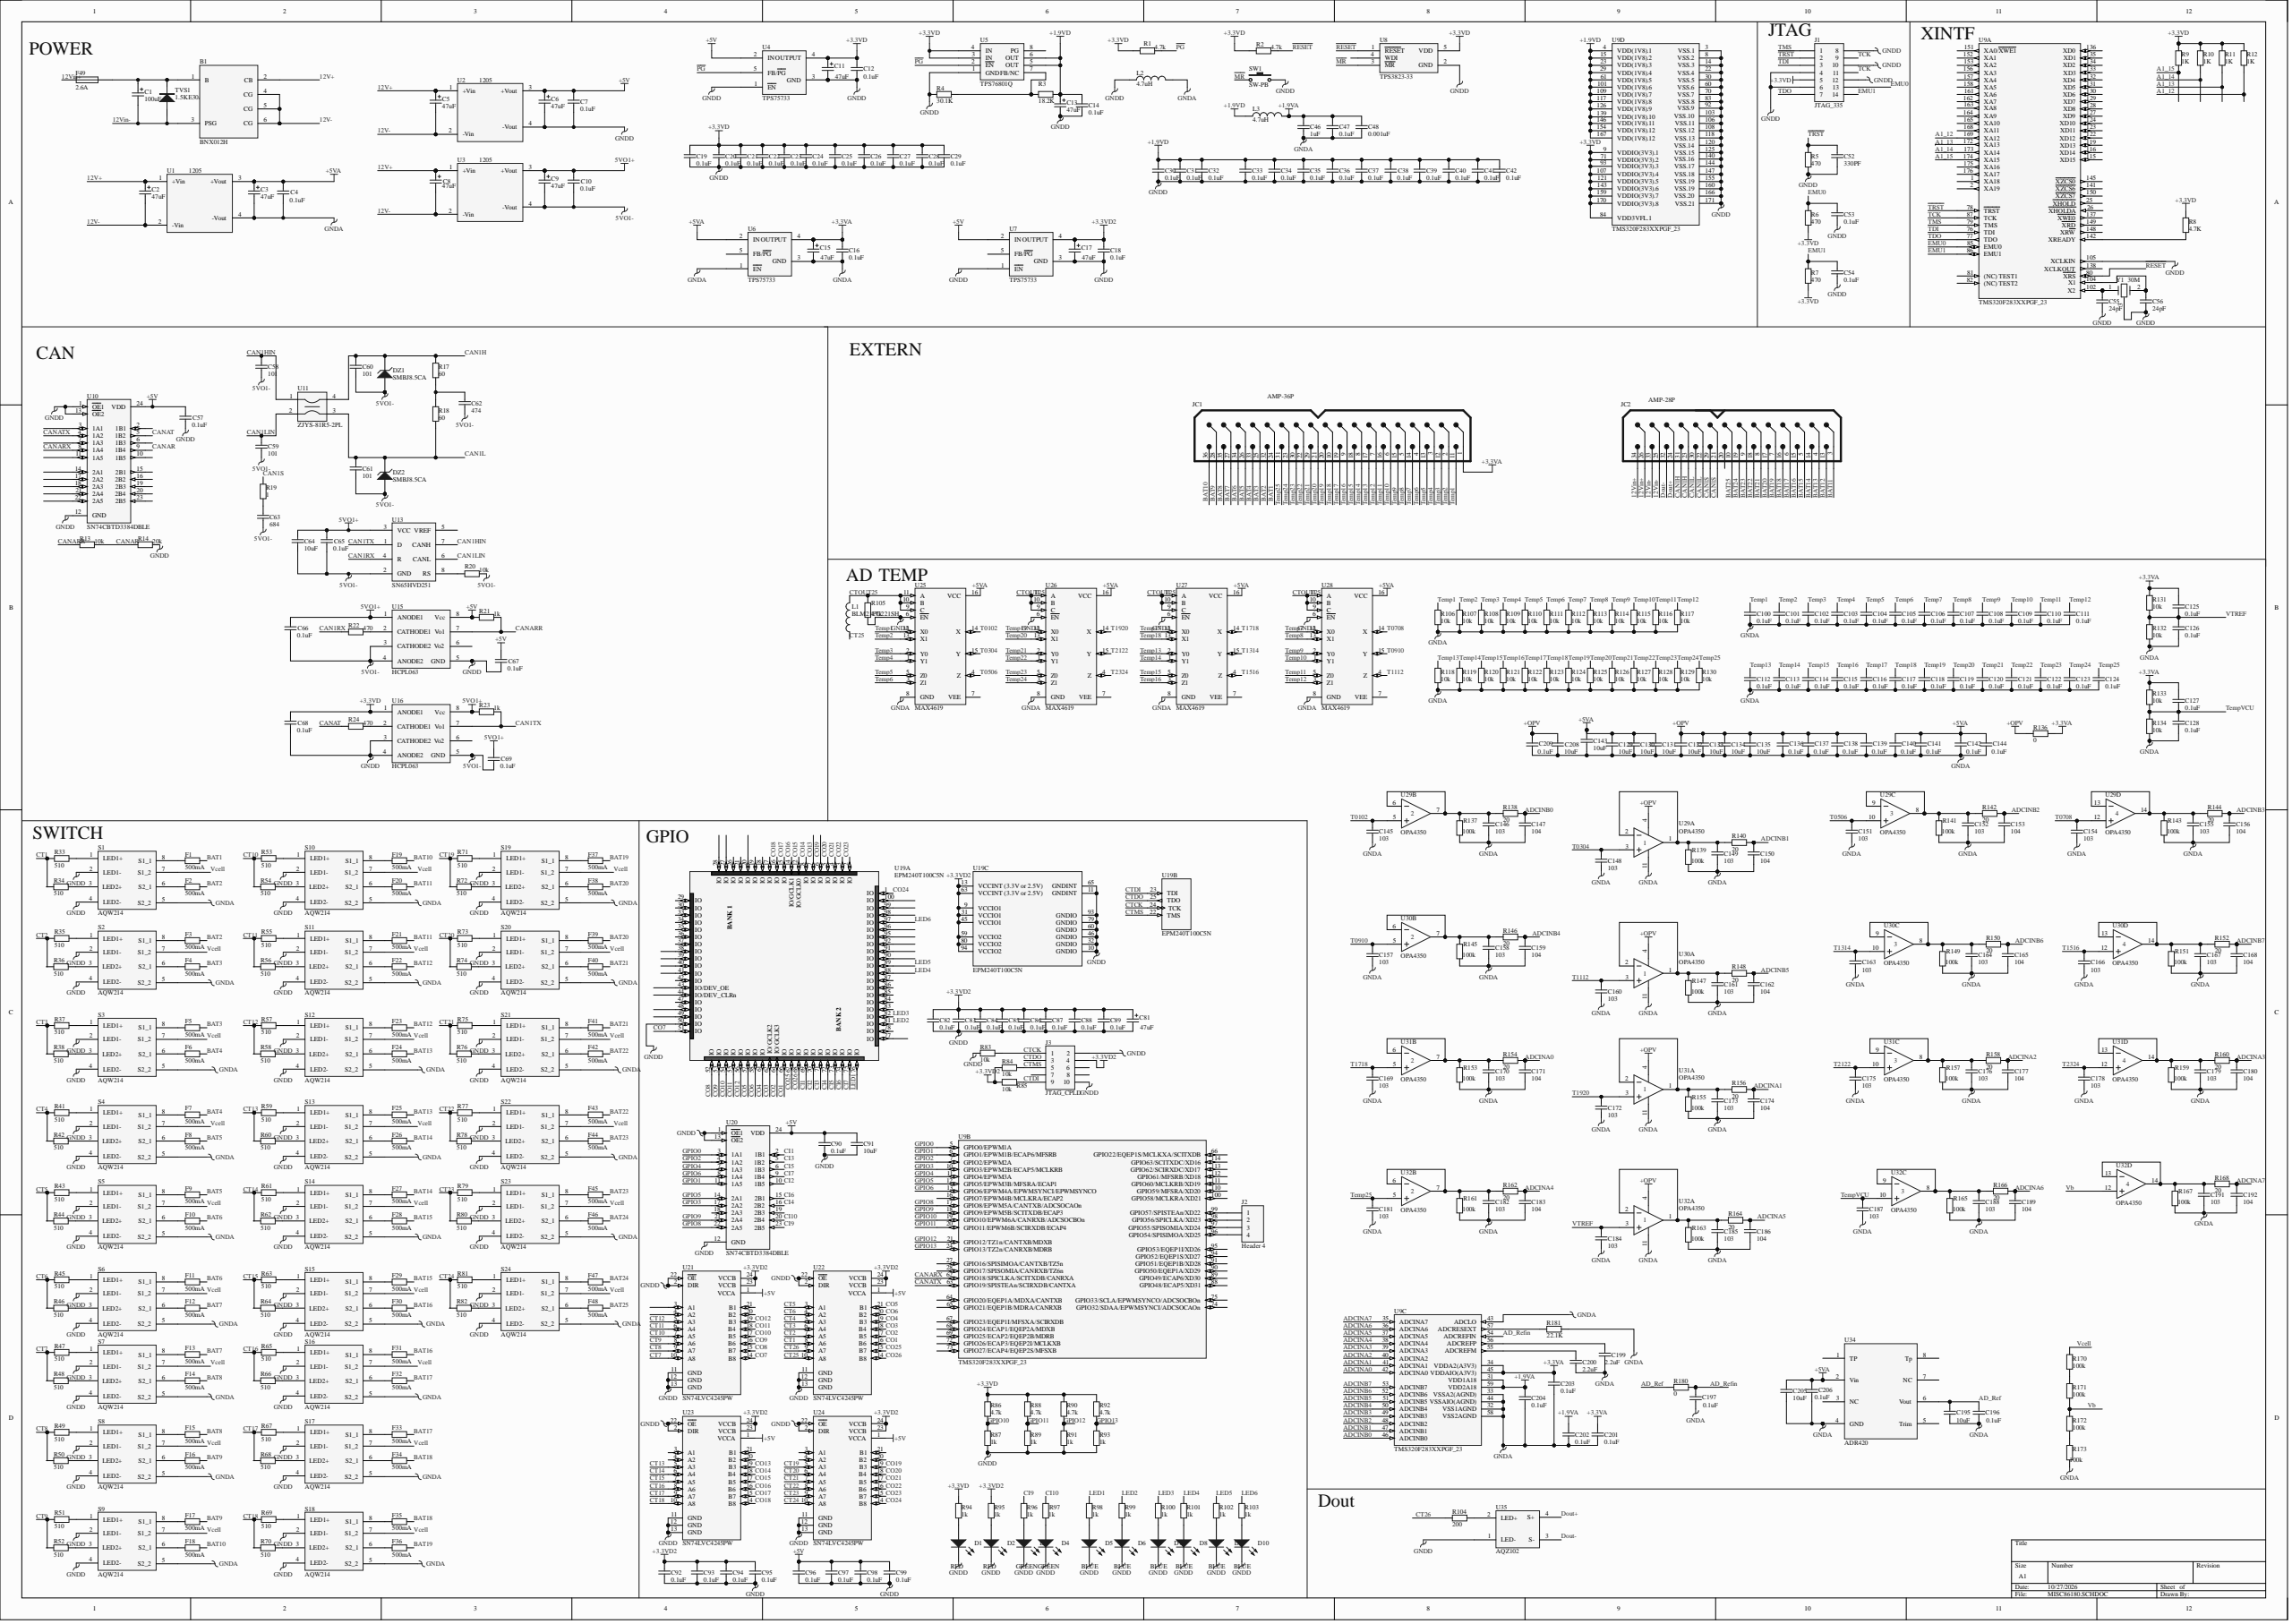Circuit board | Altium Designer | 475 parts | 355 nets
Bill of materials:
Comment,Description,Designator,Footprint,LibRef,Quantity
"BNX012H","","B1","BNX012H","BNX012H","1"
"Cap Pol3","Polarized Capacitor (Surface Mount)","C1, C2, C3, C5, C6, C8, C9, C11, C13, C15, C17, C81","TC7343-2917","Cap Pol3","12"
"Cap","Capacitor","C4, C7, C10, C125, C126, C127, C128","CR2012-0805","Cap","7"
"Cap","Capacitor","C12, C14, C16, C18, C19, C20, C21, C22, C23, C24, C25, C26, C27, C28, C29, C30, C31, C32, C33, C34, C35, C36, C37, C38, C39, C40, C41, C42, C47, C48, C52, C53, C54, C55, C56, C57, C58, C59, C60, C61, C62, C63, C65, C66, C67, C68, C69, C82, C83, C84, C85, C86, C87, C88, C89, C90, C92, C93, C94, C95, C96, C97, C98, C99, C100, C101, C102, C103, C104, C105, C106, C107, C108, C109, C110, C111, C112, C113, C114, C115, C116, C117, C118, C119, C120, C121, C122, C123, C124, C136, C137, C138, C139, C140, C141, C142, C144, C145, C146, C147, C148, C149, C150, C151, C152, C153, C154, C155, C156, C157, C158, C159, C160, C161, C162, C163, C164, C165, C166, C167, C168, C169, C170, C171, C172, C173, C174, C175, C176, C177, C178, C179, C180, C181, C182, C183, C184, C185, C186, C187, C188, C189, C191, C192, C196, C197, C199, C200, C201, C202, C203, C204, C206, C209","CR1608-0603","Cap","154"
"Cap","Capacitor","C46","1206","Cap","1"
"Cap","Capacitor","C64, C91, C129, C130, C131, C132, C133, C134, C135, C143, C195, C205, C208","CR3216-1206","Cap","13"
"RED","Typical YELLOW GaAs LED","D1, D2, D10","CR2012-0805","LED1","3"
"GREEN","Typical YELLOW GaAs LED","D3, D4","CR2012-0805","LED1","2"
"BLUE","Typical YELLOW GaAs LED","D5, D6, D7, D8, D9","CR2012-0805","LED1","5"
"SMBJ8.5CA","","DZ1, DZ2","AK_1B","AK1B","2"
"Res2","Resistor","F1, F2, F3, F4, F5, F6, F7, F8, F9, F10, F11, F12, F13, F14, F15, F16, F17, F18, F19, F20, F21, F22, F23, F24, F25, F26, F27, F28, F29, F30, F31, F32, F33, F34, F35, F36, F37, F38, F39, F40, F41, F42, F43, F44, F45, F46, F47, F48","CR6332-2512","Res2","48"
"2.6A","Fuse","F49","FUSE","FUSE1","1"
"JTAG_335","Header, 7-Pin, Dual row","J1","JTAG14","Header 7X2A","1"
"Header 4","Header, 4-Pin","J2","HDR1X4","Header 4","1"
"JTAG_CPLD","Header, 5-Pin, Dual row","J3","HDR2X5","Header 5X2","1"
"AMP-36P","","JC1","36P","AMP-36P","1"
"AMP-28P","","JC2","28P","AMP-28P","1"
"Inductor","Inductor","L1","INDC2012-0805","Inductor","1"
"Inductor","Inductor","L2, L3","CR3225-1210","Inductor","2"
"Res2","Resistor","R1, R2, R5, R6, R7, R8, R9, R10, R11, R12, R13, R14, R20, R21, R22, R23, R24, R83, R84, R85, R86, R87, R88, R89, R90, R91, R92, R93, R94, R95, R96, R97, R98, R99, R100, R101, R102, R103, R105, R137, R138, R139, R140, R141, R142, R143, R144, R145, R146, R147, R148, R149, R150, R151, R152, R153, R154, R155, R156, R157, R158, R159, R160, R161, R162, R163, R164, R165, R166, R167, R168, R181","CR1608-0603","Res2","72"
"Res2","Resistor","R3, R4, R17, R18, R19, R33, R34, R35, R36, R37, R38, R41, R42, R43, R44, R45, R46, R47, R48, R49, R50, R51, R52, R53, R54, R55, R56, R57, R58, R59, R60, R61, R62, R63, R64, R65, R66, R67, R68, R69, R70, R71, R72, R73, R74, R75, R76, R77, R78, R79, R80, R81, R82, R104, R106, R107, R108, R109, R110, R111, R112, R113, R114, R115, R116, R117, R118, R119, R120, R121, R122, R123, R124, R125, R126, R127, R128, R129, R130, R131, R132, R133, R134, R136, R170, R171, R172, R173, R180","CR2012-0805","Res2","89"
"AQW214","","S1, S2, S3, S4, S5, S6, S7, S8, S9, S10, S11, S12, S13, S14, S15, S16, S17, S18, S19, S20, S21, S22, S23, S24","AQW214","AQW214","24"
"SW-PB","Switch","SW1","SW_RESET","SW-PB","1"
"1.5KE30A","","TVS1","SB560","diode2","1"
"1205","","U1, U2, U3","DCDC_5W","DCDC","3"
"TPS75733","","U4, U6, U7","75733","TPS75733","3"
"TPS76801Q","","U5","D008","TPS76801Q","1"
"TPS3823-33","","U8","DBV005","TPS3823-33","1"
"TMS320F283XXPGF_23","","U9","QFP176NEW","TMS320F283XXPGF_23","1"
"SN74CBTD3384DBLE","10-Bit FET Bus Switch with Level Shifting","U10, U20","DBQ024","SN74CBTD3384DBLE","2"
"ZJYS-81R5-2PL","","U11","ZJYS","ZJYS-81R5-2PL","1"
"SN65HVD251","","U13","D008","SN65HVD251","1"
"HCPL063","","U15, U16","SO-G8","HCPL063","2"
"EPM240T100C5N","MAX II 2.5/3.3V CPLD, 80 I/Os, 100-Pin Plastic TQFP, Pb-Free, Commercial Temperature, Speed Grade 5","U19","TQFP100","EPM240T100C5N","1"
"SN74LVC4245PW","Octal Bus Transceiver and 3.3-V to 5-V Shifter with 3-State Outputs","U21, U22, U23, U24","WSO24","SN74LVC4245PW","4"
"MAX4619","Analog Multiplexer/Demultiplexer Triple 2-Channel","U25, U26, U27, U28","SO16","M74HC4053M1R","4"
"OPA4350","Quad Low-Power Operational Amplifier","U29, U30, U31, U32","751A-02","LM324D","4"
"ADR420","","U34","SO-G8","ADR421","1"
"AQZ102","","U35","AQZ102","AQZ","1"
"30M","Crystal","Y1","Oscillator","CRYSTAL","1"
Netlist (Protel format):
[
B1
BNX012H
BNX012H



]
[
C1
TC7343-2917
Cap Pol3



]
[
C2
TC7343-2917
Cap Pol3



]
[
C3
TC7343-2917
Cap Pol3



]
[
C4
CR2012-0805
Cap



]
[
C5
TC7343-2917
Cap Pol3



]
[
C6
TC7343-2917
Cap Pol3



]
[
C7
CR2012-0805
Cap



]
[
C8
TC7343-2917
Cap Pol3



]
[
C9
TC7343-2917
Cap Pol3



]
[
C10
CR2012-0805
Cap



]
[
C11
TC7343-2917
Cap Pol3



]
[
C12
CR1608-0603
Cap



]
[
C13
TC7343-2917
Cap Pol3



]
[
C14
CR1608-0603
Cap



]
[
C15
TC7343-2917
Cap Pol3



]
[
C16
CR1608-0603
Cap



]
[
C17
TC7343-2917
Cap Pol3



]
[
C18
CR1608-0603
Cap



]
[
C19
CR1608-0603
Cap



]
[
C20
CR1608-0603
Cap



]
[
C21
CR1608-0603
Cap



]
[
C22
CR1608-0603
Cap



]
[
C23
CR1608-0603
Cap



]
[
C24
CR1608-0603
Cap



]
[
C25
CR1608-0603
Cap



]
[
C26
CR1608-0603
Cap



]
[
C27
CR1608-0603
Cap



]
[
C28
CR1608-0603
Cap



]
[
C29
CR1608-0603
Cap



]
[
C30
CR1608-0603
Cap



]
[
C31
CR1608-0603
Cap



]
[
C32
CR1608-0603
Cap



]
[
C33
CR1608-0603
Cap



]
[
C34
CR1608-0603
Cap



]
[
C35
CR1608-0603
Cap



]
[
C36
CR1608-0603
Cap



]
[
C37
CR1608-0603
Cap



]
[
C38
CR1608-0603
Cap



]
[
C39
CR1608-0603
Cap



]
[
C40
CR1608-0603
Cap



]
[
C41
CR1608-0603
Cap



]
[
C42
CR1608-0603
Cap



]
[
C46
1206
Cap



]
[
C47
CR1608-0603
Cap



]
[
C48
CR1608-0603
Cap



]
[
C52
CR1608-0603
Cap



]
[
C53
CR1608-0603
Cap



]
[
C54
CR1608-0603
Cap



]
[
C55
CR1608-0603
Cap



]
[
C56
CR1608-0603
Cap



]
[
C57
CR1608-0603
Cap



]
[
C58
CR1608-0603
Cap



]
[
C59
CR1608-0603
Cap



]
[
C60
CR1608-0603
Cap



]
[
C61
CR1608-0603
Cap



]
[
C62
CR1608-0603
Cap



]
[
C63
CR1608-0603
Cap



]
[
C64
CR3216-1206
Cap



]
[
C65
CR1608-0603
Cap



]
[
C66
CR1608-0603
Cap



]
[
C67
CR1608-0603
Cap



]
[
C68
CR1608-0603
Cap



]
[
C69
CR1608-0603
Cap



]
[
C81
TC7343-2917
Cap Pol3



]
[
C82
CR1608-0603
Cap



]
[
C83
CR1608-0603
Cap



]
[
C84
CR1608-0603
Cap



]
[
C85
CR1608-0603
Cap



]
[
C86
CR1608-0603
Cap



]
[
C87
CR1608-0603
Cap



]
[
C88
CR1608-0603
Cap



]
[
C89
CR1608-0603
Cap



]
[
C90
CR1608-0603
Cap



]
[
C91
CR3216-1206
Cap



]
[
C92
CR1608-0603
Cap



]
[
C93
CR1608-0603
Cap



]
[
C94
CR1608-0603
Cap



]
[
C95
CR1608-0603
Cap



]
[
C96
CR1608-0603
Cap



]
[
C97
CR1608-0603
Cap



]
[
C98
CR1608-0603
Cap



]
[
C99
CR1608-0603
Cap



]
[
C100
CR1608-0603
Cap



]
[
C101
CR1608-0603
Cap



]
[
C102
CR1608-0603
Cap



]
[
C103
CR1608-0603
Cap



]
[
C104
CR1608-0603
Cap



]
[
C105
CR1608-0603
Cap



]
[
C106
CR1608-0603
Cap



]
[
C107
CR1608-0603
Cap



]
[
C108
CR1608-0603
Cap



]
[
C109
CR1608-0603
Cap



]
[
C110
CR1608-0603
Cap



]
[
C111
CR1608-0603
Cap



]
[
C112
CR1608-0603
Cap



]
[
C113
CR1608-0603
Cap



]
[
C114
CR1608-0603
Cap



]
[
C115
CR1608-0603
Cap



]
[
C116
CR1608-0603
Cap



]
[
C117
CR1608-0603
Cap



]
[
C118
CR1608-0603
Cap



]
[
C119
CR1608-0603
Cap



]
[
C120
CR1608-0603
Cap



]
[
C121
CR1608-0603
Cap



]
[
C122
CR1608-0603
Cap



]
[
C123
CR1608-0603
Cap



]
[
C124
CR1608-0603
Cap



]
[
C125
CR2012-0805
Cap



]
[
C126
CR2012-0805
Cap



]
[
C127
CR2012-0805
Cap



]
[
C128
CR2012-0805
Cap



]
[
C129
CR3216-1206
Cap



]
[
C130
CR3216-1206
Cap



]
[
C131
CR3216-1206
Cap



]
[
C132
CR3216-1206
Cap



]
[
C133
CR3216-1206
Cap



]
[
C134
CR3216-1206
Cap



]
[
C135
CR3216-1206
Cap



]
[
C136
CR1608-0603
Cap



]
[
C137
CR1608-0603
Cap



]
[
C138
CR1608-0603
Cap



]
[
C139
CR1608-0603
Cap



]
[
C140
CR1608-0603
Cap



]
[
C141
CR1608-0603
Cap



]
[
C142
CR1608-0603
Cap



]
[
C143
CR3216-1206
Cap



]
[
C144
CR1608-0603
Cap



]
[
C145
CR1608-0603
Cap



]
[
C146
CR1608-0603
Cap



]
[
C147
CR1608-0603
Cap



]
[
C148
CR1608-0603
Cap



]
[
C149
CR1608-0603
Cap



]
[
C150
CR1608-0603
Cap



]
[
C151
CR1608-0603
Cap



]
[
C152
CR1608-0603
Cap



]
[
C153
CR1608-0603
Cap



]
[
C154
CR1608-0603
Cap



]
[
C155
CR1608-0603
Cap



]
[
C156
CR1608-0603
Cap



]
[
C157
CR1608-0603
Cap



]
[
C158
CR1608-0603
Cap



]
[
C159
CR1608-0603
Cap



]
[
C160
CR1608-0603
Cap



]
[
C161
CR1608-0603
Cap



]
[
C162
CR1608-0603
Cap



]
[
C163
CR1608-0603
Cap



]
[
C164
CR1608-0603
Cap



]
[
C165
CR1608-0603
Cap



]
[
C166
CR1608-0603
Cap



]
[
C167
CR1608-0603
Cap



]
[
C168
CR1608-0603
Cap



]
[
C169
CR1608-0603
Cap



]
[
C170
CR1608-0603
Cap



]
[
C171
CR1608-0603
Cap



]
[
C172
CR1608-0603
Cap



]
[
C173
CR1608-0603
Cap



]
[
C174
CR1608-0603
Cap



]
[
C175
CR1608-0603
Cap



]
[
C176
CR1608-0603
Cap



]
[
C177
CR1608-0603
Cap



]
[
C178
CR1608-0603
Cap



]
[
C179
CR1608-0603
Cap



]
[
C180
CR1608-0603
Cap



]
[
C181
CR1608-0603
Cap



]
[
C182
CR1608-0603
Cap



]
[
C183
CR1608-0603
Cap



]
[
C184
CR1608-0603
Cap



]
[
C185
CR1608-0603
Cap



]
[
C186
CR1608-0603
Cap



]
[
C187
CR1608-0603
Cap



]
[
C188
CR1608-0603
Cap



]
[
C189
CR1608-0603
Cap



]
[
C191
CR1608-0603
Cap



]
[
C192
CR1608-0603
Cap



]
[
C195
CR3216-1206
Cap



]
[
C196
CR1608-0603
Cap



]
[
C197
CR1608-0603
Cap



]
[
C199
CR1608-0603
Cap



]
[
C200
CR1608-0603
Cap



]
[
C201
CR1608-0603
Cap



]
[
C202
CR1608-0603
Cap



]
[
C203
CR1608-0603
Cap



]
[
C204
CR1608-0603
Cap



]
[
C205
CR3216-1206
Cap



]
[
C206
CR1608-0603
Cap



]
[
C208
CR3216-1206
Cap



]
[
C209
CR1608-0603
Cap



]
[
D1
CR2012-0805
RED



]
[
D2
CR2012-0805
RED



]
[
D3
CR2012-0805
GREEN



]
[
D4
CR2012-0805
GREEN



]
[
D5
CR2012-0805
BLUE



]
[
D6
CR2012-0805
BLUE



]
[
D7
CR2012-0805
BLUE



]
[
D8
CR2012-0805
BLUE



]
[
D9
CR2012-0805
BLUE



]
[
D10
CR2012-0805
RED



]
[
DZ1
AK_1B
SMBJ8.5CA



]
[
DZ2
AK_1B
SMBJ8.5CA



]
[
F1
CR6332-2512
Res2



]
[
F2
CR6332-2512
Res2



]
[
F3
CR6332-2512
Res2



]
[
F4
CR6332-2512
Res2



]
[
F5
CR6332-2512
Res2



]
[
F6
CR6332-2512
Res2



]
[
F7
CR6332-2512
Res2



]
[
F8
CR6332-2512
Res2



]
[
F9
CR6332-2512
Res2



]
[
F10
CR6332-2512
Res2



]
[
F11
CR6332-2512
Res2



]
[
F12
CR6332-2512
Res2



]
[
F13
CR6332-2512
Res2



]
[
F14
CR6332-2512
Res2



]
[
F15
CR6332-2512
Res2



]
[
F16
CR6332-2512
Res2



]
[
F17
CR6332-2512
Res2



]
[
F18
CR6332-2512
Res2



]
[
F19
CR6332-2512
Res2



]
[
F20
CR6332-2512
Res2



]
[
F21
CR6332-2512
Res2



]
[
F22
CR6332-2512
Res2



]
[
F23
CR6332-2512
Res2



]
[
F24
CR6332-2512
Res2



]
[
F25
CR6332-2512
Res2



]
[
F26
CR6332-2512
Res2



]
[
F27
CR6332-2512
Res2



]
[
F28
CR6332-2512
Res2



]
[
F29
CR6332-2512
Res2



]
[
F30
CR6332-2512
Res2



]
[
F31
CR6332-2512
Res2



]
[
F32
CR6332-2512
Res2



]
[
F33
CR6332-2512
Res2



]
[
F34
CR6332-2512
Res2



]
[
F35
CR6332-2512
Res2



]
[
F36
CR6332-2512
Res2



]
[
F37
CR6332-2512
Res2



]
[
F38
CR6332-2512
Res2



]
[
F39
CR6332-2512
Res2



]
[
F40
CR6332-2512
Res2



]
[
F41
CR6332-2512
Res2



]
[
F42
CR6332-2512
Res2



]
[
F43
CR6332-2512
Res2



]
[
F44
CR6332-2512
Res2



]
[
F45
CR6332-2512
Res2



]
[
F46
CR6332-2512
Res2



]
[
F47
CR6332-2512
Res2



]
[
F48
CR6332-2512
Res2



]
[
F49
FUSE
2.6A



]
[
J1
JTAG14
JTAG_335



]
[
J2
HDR1X4
Header 4



]
[
J3
HDR2X5
JTAG_CPLD



]
[
JC1
36P
AMP-36P



]
[
JC2
28P
AMP-28P



]
[
L1
INDC2012-0805
Inductor



]
[
L2
CR3225-1210
Inductor



]
[
L3
CR3225-1210
Inductor



]
[
R1
CR1608-0603
Res2



]
[
R2
CR1608-0603
Res2



]
[
R3
CR2012-0805
Res2



]
[
R4
CR2012-0805
Res2



]
[
R5
CR1608-0603
Res2



]
[
R6
CR1608-0603
Res2



]
[
R7
CR1608-0603
Res2



]
[
R8
CR1608-0603
Res2



]
[
R9
CR1608-0603
Res2



]
[
R10
CR1608-0603
Res2



]
[
R11
CR1608-0603
Res2



]
[
R12
CR1608-0603
Res2



]
[
R13
CR1608-0603
Res2



]
[
R14
CR1608-0603
Res2



]
[
R17
CR2012-0805
Res2



]
[
R18
CR2012-0805
Res2



]
[
R19
CR2012-0805
Res2



]
[
R20
CR1608-0603
Res2



]
[
R21
CR1608-0603
Res2



]
[
R22
CR1608-0603
Res2



]
[
R23
CR1608-0603
Res2



]
[
R24
CR1608-0603
Res2



]
[
R33
CR2012-0805
Res2



]
[
R34
CR2012-0805
Res2



]
[
R35
CR2012-0805
Res2



]
[
R36
CR2012-0805
Res2



]
[
R37
CR2012-0805
Res2



]
[
R38
CR2012-0805
Res2



]
[
R41
CR2012-0805
Res2



]
[
R42
CR2012-0805
Res2



]
[
R43
CR2012-0805
Res2



]
[
R44
CR2012-0805
Res2



]
[
R45
CR2012-0805
Res2



]
[
R46
CR2012-0805
Res2



]
[
R47
CR2012-0805
Res2



]
[
R48
CR2012-0805
Res2



]
[
R49
CR2012-0805
Res2



]
[
R50
CR2012-0805
Res2



]
[
R51
CR2012-0805
Res2



]
[
R52
CR2012-0805
Res2



]
[
R53
CR2012-0805
Res2



]
[
R54
CR2012-0805
Res2



]
[
R55
CR2012-0805
Res2



]
[
R56
CR2012-0805
Res2



]
[
R57
CR2012-0805
Res2



]
[
R58
CR2012-0805
Res2



]
[
R59
CR2012-0805
Res2



]
[
R60
CR2012-0805
Res2



]
[
R61
CR2012-0805
Res2



]
[
R62
CR2012-0805
Res2



]
[
R63
CR2012-0805
Res2



]
[
R64
CR2012-0805
Res2



]
[
R65
CR2012-0805
Res2



]
[
R66
CR2012-0805
Res2



]
[
R67
CR2012-0805
Res2



]
[
R68
CR2012-0805
Res2



]
[
R69
CR2012-0805
Res2



]
[
R70
CR2012-0805
Res2



]
[
R71
CR2012-0805
Res2



]
[
R72
CR2012-0805
Res2



]
[
R73
CR2012-0805
Res2



]
[
R74
CR2012-0805
Res2



]
[
R75
CR2012-0805
Res2



]
[
R76
CR2012-0805
Res2



]
[
R77
CR2012-0805
Res2



]
[
R78
CR2012-0805
Res2



]
[
R79
CR2012-0805
Res2



]
[
R80
CR2012-0805
Res2



]
[
R81
CR2012-0805
Res2



]
[
R82
CR2012-0805
Res2



]
[
R83
CR1608-0603
Res2



]
[
R84
CR1608-0603
Res2



]
[
R85
CR1608-0603
Res2



]
[
R86
CR1608-0603
Res2



]
[
R87
CR1608-0603
Res2



]
[
R88
CR1608-0603
Res2



]
[
R89
CR1608-0603
Res2



]
[
R90
CR1608-0603
Res2



]
[
R91
CR1608-0603
Res2



]
[
R92
CR1608-0603
Res2



]
[
R93
CR1608-0603
Res2



]
[
R94
CR1608-0603
Res2



]
[
R95
CR1608-0603
Res2



]
[
R96
CR1608-0603
Res2



]
[
R97
CR1608-0603
Res2



]
[
R98
CR1608-0603
Res2



]
[
R99
CR1608-0603
Res2



]
[
R100
CR1608-0603
Res2



]
[
R101
CR1608-0603
Res2



]
[
R102
CR1608-0603
Res2



]
[
R103
CR1608-0603
Res2



]
[
R104
CR2012-0805
Res2



]
[
R105
CR1608-0603
Res2



]
[
R106
CR2012-0805
Res2



]
[
R107
CR2012-0805
Res2



]
[
R108
CR2012-0805
Res2



]
[
R109
CR2012-0805
Res2



]
[
R110
CR2012-0805
Res2



]
[
R111
CR2012-0805
Res2



]
[
R112
CR2012-0805
Res2



]
[
R113
CR2012-0805
Res2



]
[
R114
CR2012-0805
Res2



]
[
R115
CR2012-0805
Res2



]
[
R116
CR2012-0805
Res2



]
[
R117
CR2012-0805
Res2



]
[
R118
CR2012-0805
Res2



]
[
R119
CR2012-0805
Res2



]
[
R120
CR2012-0805
Res2



]
[
R121
CR2012-0805
Res2



]
[
R122
CR2012-0805
Res2



]
[
R123
CR2012-0805
Res2



]
[
R124
CR2012-0805
Res2



]
[
R125
CR2012-0805
Res2



]
[
R126
CR2012-0805
Res2



]
[
R127
CR2012-0805
Res2



]
[
R128
CR2012-0805
Res2



]
[
R129
CR2012-0805
Res2



]
[
R130
CR2012-0805
Res2



]
[
R131
CR2012-0805
Res2



]
[
R132
CR2012-0805
Res2



]
[
R133
CR2012-0805
Res2



]
[
R134
CR2012-0805
Res2



]
[
R136
CR2012-0805
Res2



]
[
R137
CR1608-0603
Res2



]
[
R138
CR1608-0603
Res2



]
[
R139
CR1608-0603
Res2



]
[
R140
CR1608-0603
Res2



]
[
R141
CR1608-0603
Res2



]
[
R142
CR1608-0603
Res2



]
[
R143
CR1608-0603
Res2



]
[
R144
CR1608-0603
Res2



]
[
R145
CR1608-0603
Res2



]
[
R146
CR1608-0603
Res2



]
[
R147
CR1608-0603
Res2



]
[
R148
CR1608-0603
Res2



]
[
R149
CR1608-0603
Res2



]
[
R150
CR1608-0603
Res2



]
[
R151
CR1608-0603
Res2



]
[
R152
CR1608-0603
Res2



]
[
R153
CR1608-0603
Res2



]
[
R154
CR1608-0603
Res2



]
[
R155
CR1608-0603
Res2



]
[
R156
CR1608-0603
Res2



]
[
R157
CR1608-0603
Res2



]
[
R158
CR1608-0603
Res2



]
[
R159
CR1608-0603
Res2



]
[
R160
CR1608-0603
Res2



]
[
R161
CR1608-0603
Res2



]
[
R162
CR1608-0603
Res2



]
[
R163
CR1608-0603
Res2



]
[
R164
CR1608-0603
Res2



]
[
R165
CR1608-0603
Res2



]
[
R166
CR1608-0603
Res2



]
[
R167
CR1608-0603
Res2



]
[
R168
CR1608-0603
Res2



]
[
R170
CR2012-0805
Res2



]
[
R171
CR2012-0805
Res2



]
[
R172
CR2012-0805
Res2



]
[
R173
CR2012-0805
Res2



]
[
R180
CR2012-0805
Res2



]
[
R181
CR1608-0603
Res2



]
[
S1
AQW214
AQW214



]
[
S2
AQW214
AQW214



]
[
S3
AQW214
AQW214



]
[
S4
AQW214
AQW214



]
[
S5
AQW214
AQW214



]
[
S6
AQW214
AQW214



]
[
S7
AQW214
AQW214



]
[
S8
AQW214
AQW214



]
[
S9
AQW214
AQW214



]
[
S10
AQW214
AQW214



]
[
S11
AQW214
AQW214



]
[
S12
AQW214
AQW214



]
[
S13
AQW214
AQW214



]
[
S14
AQW214
AQW214



]
[
S15
AQW214
AQW214



]
[
S16
AQW214
AQW214



]
[
S17
AQW214
AQW214



]
[
S18
AQW214
AQW214



]
[
S19
AQW214
AQW214



]
[
S20
AQW214
AQW214



]
[
S21
AQW214
AQW214



]
[
S22
AQW214
AQW214



]
[
S23
AQW214
AQW214



]
[
S24
AQW214
AQW214



]
[
SW1
SW_RESET
SW-PB



]
[
TVS1
SB560
1.5KE30A



]
[
U1
DCDC_5W
1205



]
[
U2
DCDC_5W
1205



]
[
U3
DCDC_5W
1205



]
[
U4
75733
TPS75733



]
[
U5
D008
TPS76801Q



]
[
U6
75733
TPS75733



]
[
U7
75733
TPS75733



]
[
U8
DBV005
TPS3823-33



]
[
U9
QFP176NEW
TMS320F283XXPGF_23



]
[
U10
DBQ024
SN74CBTD3384DBLE



]
[
U11
ZJYS
ZJYS-81R5-2PL



]
[
U13
D008
SN65HVD251



]
[
U15
SO-G8
HCPL063



]
[
U16
SO-G8
HCPL063



]
[
U19
TQFP100
EPM240T100C5N



]
[
U20
DBQ024
SN74CBTD3384DBLE



]
[
U21
WSO24
SN74LVC4245PW



]
[
U22
WSO24
SN74LVC4245PW



]
[
U23
WSO24
SN74LVC4245PW



]
[
U24
WSO24
SN74LVC4245PW



]
[
U25
SO16
MAX4619



]
[
U26
SO16
MAX4619



]
[
U27
SO16
MAX4619



]
[
U28
SO16
MAX4619



]
[
U29
751A-02
OPA4350



]
[
U30
751A-02
OPA4350



]
[
U31
751A-02
OPA4350



]
[
U32
751A-02
OPA4350



]
[
U34
SO-G8
ADR420



]
[
U35
AQZ102
AQZ102



]
[
Y1
Oscillator
30M



]
(
VTREF
C125-1
C126-2
C184-2
R131-2
R132-1
U32-3
)
(
Vcell
R170-1
S1-7
S2-7
S3-7
S4-7
S5-7
S6-7
S7-7
S8-7
S9-7
S10-7
S11-7
S12-7
S13-7
S14-7
S15-7
S16-7
S17-7
S18-7
S19-7
S20-7
S21-7
S22-7
S23-7
S24-7
)
(
Vb
R171-2
R172-1
U32-12
)
(
TMS
J1-1
U9-79
)
(
TempVCU
C127-1
C128-2
C187-2
R133-2
R134-1
U32-10
)
(
Temp25
C124-2
C181-2
JC1-31
R130-1
U32-5
)
(
Temp24
C123-2
JC1-23
R129-1
U26-3
)
(
Temp23
C122-2
JC1-30
R128-1
U26-5
)
(
Temp22
C121-2
JC1-22
R127-1
U26-1
)
(
Temp21
C120-2
JC1-29
R126-1
U26-2
)
(
Temp20
C119-2
JC1-21
R125-1
U26-13
)
(
Temp19
C118-2
JC1-20
R124-1
U26-12
)
(
Temp18
C117-2
JC1-10
R123-1
U27-13
)
(
Temp17
C116-2
JC1-19
R122-1
U27-12
)
(
Temp16
C115-2
JC1-9
R121-1
U27-3
)
(
Temp15
C114-2
JC1-18
R120-1
U27-5
)
(
Temp14
C113-2
JC1-8
R119-1
U27-1
)
(
Temp13
C112-2
JC1-17
R118-1
U27-2
)
(
Temp12
C111-2
JC1-7
R117-1
U28-3
)
(
Temp11
C110-2
JC1-16
R116-1
U28-5
)
(
Temp10
C109-2
JC1-6
R115-1
U28-1
)
(
Temp9
C108-2
JC1-15
R114-1
U28-2
)
(
Temp8
C107-2
JC1-5
R113-1
U28-13
)
(
Temp7
C106-2
JC1-14
R112-1
U28-12
)
(
Temp6
C105-2
JC1-4
R111-1
U25-3
)
(
Temp5
C104-2
JC1-13
R110-1
U25-5
)
(
Temp4
C103-2
JC1-3
R109-1
U25-1
)
(
Temp3
C102-2
JC1-12
R108-1
U25-2
)
(
Temp2
C101-2
JC1-2
R107-1
U25-13
)
(
Temp1
C100-2
JC1-11
R106-1
U25-12
)
(
TDO
J1-7
U9-77
)
(
TDI
J1-3
U9-76
)
(
TCK
J1-9
J1-11
U9-87
)
(
T\R\S\T\
C52-2
J1-2
R5-2
U9-78
)
(
T2324
C178-2
U26-4
U31-12
)
(
T2122
C175-2
U26-15
U31-10
)
(
T1920
C172-2
U26-14
U31-3
)
(
T1718
C169-2
U27-14
U31-5
)
(
T1516
C166-2
U27-4
U30-12
)
(
T1314
C163-2
U27-15
U30-10
)
(
T1112
C160-2
U28-4
U30-3
)
(
T0910
C157-2
U28-15
U30-5
)
(
T0708
C154-2
U28-14
U29-12
)
(
T0506
C151-2
U25-4
U29-10
)
(
T0304
C148-2
U25-15
U29-3
)
(
T0102
C145-2
U25-14
U29-5
)
(
R\E\S\E\T\
R2-2
U8-1
U9-80
)
(
P\G\
R1-2
U4-5
U5-2
)
(
NetR181_1
R181-1
U9-57
)
(
NetR172_2
R172-2
R173-1
)
(
NetR170_2
R170-2
R171-1
)
(
NetR104_1
R104-1
U35-2
)
(
NetR82_1
R82-1
S24-3
)
(
NetR81_1
R81-1
S24-1
)
(
NetR80_1
R80-1
S23-3
)
(
NetR79_1
R79-1
S23-1
)
(
NetR78_1
R78-1
S22-3
)
(
NetR77_1
R77-1
S22-1
)
(
NetR76_1
R76-1
S21-3
)
(
NetR75_1
R75-1
S21-1
)
(
NetR74_1
R74-1
S20-3
)
(
NetR73_1
R73-1
S20-1
)
(
NetR72_1
R72-1
S19-3
)
(
NetR71_1
R71-1
S19-1
)
(
NetR70_1
R70-1
S18-3
)
(
NetR69_1
R69-1
S18-1
)
(
NetR68_1
R68-1
S17-3
)
(
NetR67_1
R67-1
S17-1
)
(
NetR66_1
R66-1
S16-3
)
(
NetR65_1
R65-1
S16-1
)
(
NetR64_1
R64-1
S15-3
)
(
NetR63_1
R63-1
S15-1
)
(
NetR62_1
R62-1
S14-3
)
(
NetR61_1
R61-1
S14-1
)
(
NetR60_1
R60-1
S13-3
)
(
NetR59_1
R59-1
S13-1
)
(
NetR58_1
R58-1
S12-3
)
(
NetR57_1
R57-1
S12-1
)
(
NetR56_1
R56-1
S11-3
)
(
NetR55_1
R55-1
S11-1
)
(
NetR54_1
R54-1
S10-3
)
(
NetR53_1
R53-1
S10-1
)
(
NetR52_1
R52-1
S9-3
)
(
NetR51_1
R51-1
S9-1
)
(
NetR50_1
R50-1
S8-3
)
(
NetR49_1
R49-1
S8-1
)
(
NetR48_1
R48-1
S7-3
)
(
NetR47_1
R47-1
S7-1
)
(
NetR46_1
R46-1
S6-3
)
(
NetR45_1
R45-1
S6-1
)
(
NetR44_1
R44-1
S5-3
)
(
NetR43_1
R43-1
S5-1
)
(
NetR42_1
R42-1
S4-3
)
(
NetR41_1
R41-1
S4-1
)
(
NetR38_1
R38-1
S3-3
)
(
NetR37_1
R37-1
S3-1
)
(
NetR36_1
R36-1
S2-3
)
(
NetR35_1
R35-1
S2-1
)
(
NetR34_1
R34-1
S1-3
)
(
NetR33_1
R33-1
S1-1
)
(
NetR24_1
R24-1
U16-2
)
(
NetR22_1
R22-1
U15-2
)
(
NetR20_2
R20-2
U13-8
)
(
NetR8_1
R8-1
U9-142
)
(
NetR3_1
R3-1
R4-2
U5-7
)
(
NetJ2_4
J2-4
U9-96
)
(
NetJ2_3
J2-3
U9-97
)
(
NetJ2_2
J2-2
U9-98
)
(
NetJ2_1
J2-1
U9-99
)
(
NetF48_2
F48-2
S24-6
)
(
NetF47_2
F47-2
S24-8
)
(
NetF46_2
F46-2
S23-6
)
(
NetF45_2
F45-2
S23-8
)
(
NetF44_2
F44-2
S22-6
)
(
NetF43_2
F43-2
S22-8
)
(
NetF42_2
F42-2
S21-6
)
(
NetF41_2
F41-2
S21-8
)
(
NetF40_2
F40-2
S20-6
)
(
NetF39_2
F39-2
S20-8
)
(
NetF38_2
F38-2
S19-6
)
(
NetF37_2
F37-2
S19-8
)
(
NetF36_2
F36-2
S18-6
)
(
NetF35_2
F35-2
S18-8
)
(
NetF34_2
F34-2
S17-6
)
(
NetF33_2
F33-2
S17-8
)
(
NetF32_2
F32-2
S16-6
)
(
NetF31_2
F31-2
S16-8
)
(
NetF30_2
F30-2
S15-6
)
(
NetF29_2
F29-2
S15-8
)
(
NetF28_2
F28-2
S14-6
)
(
NetF27_2
F27-2
S14-8
)
(
NetF26_2
F26-2
S13-6
)
(
NetF25_2
F25-2
S13-8
)
(
NetF24_2
F24-2
S12-6
)
(
NetF23_2
F23-2
S12-8
)
(
NetF22_2
F22-2
S11-6
)
(
NetF21_2
F21-2
S11-8
)
(
NetF20_2
F20-2
S10-6
)
(
NetF19_2
F19-2
S10-8
)
(
NetF18_2
F18-2
S9-6
)
(
NetF17_2
F17-2
S9-8
)
(
NetF16_2
F16-2
S8-6
)
(
NetF15_2
F15-2
S8-8
)
(
NetF14_2
F14-2
S7-6
)
(
NetF13_2
F13-2
S7-8
)
(
NetF12_2
F12-2
S6-6
)
(
NetF11_2
F11-2
S6-8
)
(
NetF10_2
F10-2
S5-6
)
(
NetF9_2
F9-2
S5-8
)
(
NetF8_2
F8-2
S4-6
)
(
NetF7_2
F7-2
S4-8
)
(
NetF6_2
F6-2
S3-6
)
(
NetF5_2
F5-2
S3-8
)
(
NetF4_2
F4-2
S2-6
)
(
NetF3_2
F3-2
S2-8
)
(
NetF2_2
F2-2
S1-6
)
(
NetF1_2
F1-2
S1-8
)
(
NetD10_1
D10-1
R103-2
)
(
NetD9_1
D9-1
R102-2
)
(
NetD8_1
D8-1
R101-2
)
(
NetD7_1
D7-1
R100-2
)
(
NetD6_1
D6-1
R99-2
)
(
NetD5_1
D5-1
R98-2
)
(
NetD4_1
D4-1
R97-2
)
(
NetD3_1
D3-1
R96-2
)
(
NetD2_1
D2-1
R95-2
)
(
NetD1_1
D1-1
R94-2
)
(
NetC200_2
C200-2
U9-55
)
(
NetC199_2
C199-2
U9-56
)
(
NetC191_2
C191-2
R167-2
R168-2
U32-13
U32-14
)
(
NetC188_2
C188-2
R165-2
R166-2
U32-8
U32-9
)
(
NetC185_2
C185-2
R163-2
R164-2
U32-1
U32-2
)
(
NetC182_2
C182-2
R161-2
R162-2
U32-6
U32-7
)
(
NetC179_2
C179-2
R159-2
R160-2
U31-13
U31-14
)
(
NetC176_2
C176-2
R157-2
R158-2
U31-8
U31-9
)
(
NetC173_2
C173-2
R155-2
R156-2
U31-1
U31-2
)
(
NetC170_2
C170-2
R153-2
R154-2
U31-6
U31-7
)
(
NetC167_2
C167-2
R151-2
R152-2
U30-13
U30-14
)
(
NetC164_2
C164-2
R149-2
R150-2
U30-8
U30-9
)
(
NetC161_2
C161-2
R147-2
R148-2
U30-1
U30-2
)
(
NetC158_2
C158-2
R145-2
R146-2
U30-6
U30-7
)
(
NetC155_2
C155-2
R143-2
R144-2
U29-13
U29-14
)
(
NetC152_2
C152-2
R141-2
R142-2
U29-8
U29-9
)
(
NetC149_2
C149-2
R139-2
R140-2
U29-1
U29-2
)
(
NetC146_2
C146-2
R137-2
R138-2
U29-6
U29-7
)
(
NetC63_2
C63-2
R19-1
)
(
NetC62_2
C62-2
R17-1
R18-2
)
(
NetC56_2
C56-2
U9-104
Y1-2
)
(
NetC55_2
C55-2
U9-102
Y1-1
)
(
NetB1_1
B1-1
C1-1
F49-1
TVS1-2
)
(
M\R\
SW1-1
U8-3
)
(
LED6
R103-1
U19-97
)
(
LED5
R102-1
U19-89
)
(
LED4
R101-1
U19-88
)
(
LED3
R100-1
U19-82
)
(
LED2
R99-1
U19-81
)
(
LED1
R98-1
U19-76
)
(
GPIO13
R92-2
R93-1
U9-24
)
(
GPIO12
R90-2
R91-1
U9-21
)
(
GPIO11
R88-2
R89-1
U9-20
)
(
GPIO10
R86-2
R87-1
U9-19
)
(
GPIO9
U9-18
U20-21
)
(
GPIO8
U9-17
U20-22
)
(
GPIO6
U9-13
U20-8
)
(
GPIO5
U9-12
U20-14
)
(
GPIO4
U9-11
U20-7
)
(
GPIO3
U9-10
U20-17
)
(
GPIO2
U9-7
U20-4
)
(
GPIO1
U9-6
U20-11
)
(
GPIO0
U9-5
U20-3
)
(
GNDD
C6-2
C7-1
C11-2
C12-1
C13-2
C14-1
C17-2
C18-1
C19-1
C20-1
C21-1
C22-1
C23-1
C24-1
C25-1
C26-1
C27-1
C28-1
C29-1
C30-1
C31-1
C32-1
C33-1
C34-1
C35-1
C36-1
C37-1
C38-1
C39-1
C40-1
C41-1
C42-1
C52-1
C53-1
C54-1
C55-1
C56-1
C57-1
C67-1
C68-1
C81-2
C82-1
C83-1
C84-1
C85-1
C86-1
C87-1
C88-1
C89-1
C90-1
C91-1
C92-1
C93-1
C94-1
C95-1
C96-1
C97-1
C98-1
C99-1
D1-2
D2-2
D3-2
D4-2
D5-2
D6-2
D7-2
D8-2
D9-2
D10-2
J1-4
J1-6
J1-8
J1-10
J1-12
J3-2
J3-10
L2-1
R4-1
R5-1
R14-1
R83-1
R87-2
R89-2
R91-2
R93-2
S1-2
S1-4
S2-2
S2-4
S3-2
S3-4
S4-2
S4-4
S5-2
S5-4
S6-2
S6-4
S7-2
S7-4
S8-2
S8-4
S9-2
S9-4
S10-2
S10-4
S11-2
S11-4
S12-2
S12-4
S13-2
S13-4
S14-2
S14-4
S15-2
S15-4
S16-2
S16-4
S17-2
S17-4
S18-2
S18-4
S19-2
S19-4
S20-2
S20-4
S21-2
S21-4
S22-2
S22-4
S23-2
S23-4
S24-2
S24-4
SW1-2
U2-4
U4-1
U4-3
U5-1
U7-1
U7-3
U8-2
U9-3
U9-8
U9-14
U9-22
U9-30
U9-60
U9-70
U9-83
U9-92
U9-103
U9-105
U9-106
U9-108
U9-118
U9-120
U9-125
U9-140
U9-144
U9-147
U9-155
U9-160
U9-166
U9-171
U10-1
U10-12
U10-13
U15-5
U16-3
U16-4
U19-10
U19-11
U19-32
U19-46
U19-50
U19-60
U19-65
U19-79
U19-93
U20-1
U20-12
U20-13
U21-2
U21-11
U21-12
U21-13
U21-22
U22-2
U22-11
U22-12
U22-13
U22-22
U23-2
U23-11
U23-12
U23-13
U23-22
U24-2
U24-11
U24-12
U24-13
U24-22
U35-1
Y1-3
)
(
GNDA
C3-2
C4-1
C15-2
C16-1
C46-1
C47-1
C48-1
C100-1
C101-1
C102-1
C103-1
C104-1
C105-1
C106-1
C107-1
C108-1
C109-1
C110-1
C111-1
C112-1
C113-1
C114-1
C115-1
C116-1
C117-1
C118-1
C119-1
C120-1
C121-1
C122-1
C123-1
C124-1
C126-1
C128-1
C129-1
C130-1
C131-1
C132-1
C133-1
C134-1
C135-1
C136-1
C137-1
C138-1
C139-1
C140-1
C141-1
C142-1
C143-1
C144-1
C145-1
C146-1
C147-1
C148-1
C149-1
C150-1
C151-1
C152-1
C153-1
C154-1
C155-1
C156-1
C157-1
C158-1
C159-1
C160-1
C161-1
C162-1
C163-1
C164-1
C165-1
C166-1
C167-1
C168-1
C169-1
C170-1
C171-1
C172-1
C173-1
C174-1
C175-1
C176-1
C177-1
C178-1
C179-1
C180-1
C181-1
C182-1
C183-1
C184-1
C185-1
C186-1
C187-1
C188-1
C189-1
C191-1
C192-1
C195-1
C196-1
C197-1
C199-1
C200-1
C201-1
C202-1
C203-1
C204-1
C205-1
C206-1
C208-1
C209-1
L2-2
R105-1
R106-2
R107-2
R108-2
R109-2
R110-2
R111-2
R112-2
R113-2
R114-2
R115-2
R116-2
R117-2
R118-2
R119-2
R120-2
R121-2
R122-2
R123-2
R124-2
R125-2
R126-2
R127-2
R128-2
R129-2
R130-2
R132-2
R134-2
R137-1
R139-1
R141-1
R143-1
R145-1
R147-1
R149-1
R151-1
R153-1
R155-1
R157-1
R159-1
R161-1
R163-1
R165-1
R167-1
R173-2
R181-2
S1-5
S2-5
S3-5
S4-5
S5-5
S6-5
S7-5
S8-5
S9-5
S10-5
S11-5
S12-5
S13-5
S14-5
S15-5
S16-5
S17-5
S18-5
S19-5
S20-5
S21-5
S22-5
S23-5
S24-5
U1-4
U6-1
U6-3
U9-32
U9-33
U9-43
U9-44
U9-58
U25-6
U25-8
U26-6
U26-8
U27-6
U27-8
U28-6
U28-8
U29-11
U30-11
U31-11
U32-11
U34-4
)
(
EMU1
C54-2
J1-14
R7-2
U9-86
)
(
EMU0
C53-2
J1-13
R6-2
U9-85
)
(
Dout-
JC2-32
U35-3
)
(
Dout+
JC2-24
U35-4
)
(
CTOUT25
L1-2
R105-2
U25-9
U25-10
U25-11
U26-9
U26-10
U26-11
U27-9
U27-10
U27-11
U28-9
U28-10
U28-11
)
(
CTMS
J3-5
R84-2
U19-22
)
(
CTDO
J3-3
U19-25
)
(
CTDI
J3-9
R85-2
U19-23
)
(
CTCK
J3-1
R83-2
U19-24
)
(
CT26
R104-2
U22-9
)
(
CT25
L1-1
U22-10
)
(
CT24
R81-2
R82-2
U24-10
)
(
CT23
R79-2
R80-2
U24-9
)
(
CT22
R77-2
R78-2
U24-8
)
(
CT21
R75-2
R76-2
U24-7
)
(
CT20
R73-2
R74-2
U24-6
)
(
CT19
R71-2
R72-2
U24-5
)
(
CT18
R69-2
R70-2
U23-10
)
(
CT17
R67-2
R68-2
U23-9
)
(
CT16
R65-2
R66-2
U23-8
)
(
CT15
R63-2
R64-2
U23-7
)
(
CT14
R61-2
R62-2
U23-6
)
(
CT13
R59-2
R60-2
U23-5
)
(
CT12
R57-2
R58-2
U21-5
)
(
CT11
R55-2
R56-2
U21-6
)
(
CT10
R53-2
R54-2
U21-7
)
(
CT9
R51-2
R52-2
U21-8
)
(
CT8
R49-2
R50-2
U21-9
)
(
CT7
R47-2
R48-2
U21-10
)
(
CT6
R45-2
R46-2
U22-4
)
(
CT5
R43-2
R44-2
U22-3
)
(
CT4
R41-2
R42-2
U22-5
)
(
CT3
R37-2
R38-2
U22-6
)
(
CT2
R35-2
R36-2
U22-7
)
(
CT1
R33-2
R34-2
U22-8
)
(
CO26
U19-68
U22-14
)
(
CO25
U19-67
U22-15
)
(
CO24
U19-1
U24-14
)
(
CO23
U19-2
U24-15
)
(
CO22
U19-3
U24-16
)
(
CO21
U19-4
U24-17
)
(
CO20
U19-5
U24-18
)
(
CO19
U19-6
U24-19
)
(
CO18
U19-16
U23-14
)
(
CO17
U19-15
U23-15
)
(
CO16
U19-14
U23-16
)
(
CO15
U19-12
U23-17
)
(
CO14
U19-8
U23-18
)
(
CO13
U19-7
U23-19
)
(
CO12
U19-56
U21-19
)
(
CO11
U19-55
U21-18
)
(
CO10
U19-54
U21-17
)
(
CO9
U19-53
U21-16
)
(
CO8
U19-52
U21-15
)
(
CO7
U19-51
U21-14
)
(
CO6
U19-58
U22-20
)
(
CO5
U19-57
U22-21
)
(
CO4
U19-61
U22-19
)
(
CO3
U19-62
U22-18
)
(
CO2
U19-64
U22-17
)
(
CO1
U19-66
U22-16
)
(
CI10
R97-1
U20-20
)
(
CI9
R96-1
U20-23
)
(
CI7
U19-75
U20-9
)
(
CI6
U19-74
U20-15
)
(
CI5
U19-73
U20-6
)
(
CI4
U19-72
U20-16
)
(
CI3
U19-71
U20-5
)
(
CI2
U19-70
U20-10
)
(
CI1
U19-69
U20-2
)
(
CANATX
U9-63
U10-4
)
(
CANAT
R24-2
U10-5
)
(
CANARX
U9-62
U10-8
)
(
CANARR
R13-2
R21-1
U15-7
)
(
CANAR
R13-1
R14-2
U10-9
)
(
CAN1TX
R23-1
U13-1
U16-7
)
(
CAN1S
JC2-21
JC2-29
R19-2
)
(
CAN1RX
R22-2
U13-4
)
(
CAN1LIN
C59-2
U11-2
U13-6
)
(
CAN1L
C61-2
DZ2-1
JC2-22
JC2-30
R18-1
U11-3
)
(
CAN1HIN
C58-2
U11-1
U13-7
)
(
CAN1H
C60-2
DZ1-1
JC2-23
JC2-31
R17-2
U11-4
)
(
BAT25
F48-1
JC2-10
)
(
BAT24
F46-1
F47-1
JC2-19
)
(
BAT23
F44-1
F45-1
JC2-9
)
(
BAT22
F42-1
F43-1
JC2-18
)
(
BAT21
F40-1
F41-1
JC2-8
)
(
BAT20
F38-1
F39-1
JC2-17
)
(
BAT19
F36-1
F37-1
JC2-7
)
(
BAT18
F34-1
F35-1
JC2-16
)
(
BAT17
F32-1
F33-1
JC2-6
)
(
BAT16
F30-1
F31-1
JC2-15
)
(
BAT15
F28-1
F29-1
JC2-5
)
(
BAT14
F26-1
F27-1
JC2-14
)
(
BAT13
F24-1
F25-1
JC2-4
)
(
BAT12
F22-1
F23-1
JC2-13
)
(
BAT11
F20-1
F21-1
JC2-3
)
(
BAT10
F18-1
F19-1
JC1-36
)
(
BAT9
F16-1
F17-1
JC1-28
)
(
BAT8
F14-1
F15-1
JC1-35
)
(
BAT7
F12-1
F13-1
JC1-27
)
(
BAT6
F10-1
F11-1
JC1-34
)
(
BAT5
F8-1
F9-1
JC1-26
)
(
BAT4
F6-1
F7-1
JC1-33
)
(
BAT3
F4-1
F5-1
JC1-25
)
(
BAT2
F2-1
F3-1
JC1-32
)
(
BAT1
F1-1
JC1-24
)
(
ADCINB7
C168-2
R152-1
U9-53
)
(
ADCINB6
C165-2
R150-1
U9-52
)
(
ADCINB5
C162-2
R148-1
U9-51
)
(
ADCINB4
C159-2
R146-1
U9-50
)
(
ADCINB3
C156-2
R144-1
U9-49
)
(
ADCINB2
C153-2
R142-1
U9-48
)
(
ADCINB1
C150-2
R140-1
U9-47
)
(
ADCINB0
C147-2
R138-1
U9-46
)
(
ADCINA7
C192-2
R168-1
U9-35
)
(
ADCINA6
C189-2
R166-1
U9-36
)
(
ADCINA5
C186-2
R164-1
U9-37
)
(
ADCINA4
C183-2
R162-1
U9-38
)
(
ADCINA3
C180-2
R160-1
U9-39
)
(
ADCINA2
C177-2
R158-1
U9-40
)
(
ADCINA1
C174-2
R156-1
U9-41
)
(
ADCINA0
C171-2
R154-1
U9-42
)
(
AD_Refin
C197-2
R180-1
U9-54
)
(
AD_Ref
C195-2
C196-2
R180-2
U34-6
)
(
A1_15
R9-1
U9-174
)
(
A1_14
R10-1
U9-173
)
(
A1_13
R11-1
U9-172
)
(
A1_12
R12-1
U9-169
)
(
+OPV
C132-2
C133-2
C134-2
C135-2
C136-2
C137-2
C138-2
C139-2
C208-2
C209-2
R136-2
U29-4
U30-4
U31-4
U32-4
)
(
+5VA
C3-1
C4-2
C129-2
C130-2
C131-2
C140-2
C141-2
C142-2
C143-2
C144-2
C205-2
C206-2
U1-3
U6-2
U25-16
U26-16
U27-16
U28-16
U34-2
)
(
+5V
C6-1
C7-2
C57-2
C67-2
C90-2
C91-2
C96-2
C97-2
C98-2
C99-2
R21-2
U2-3
U4-2
U7-2
U10-24
U15-8
U20-24
U21-1
U22-1
U23-1
U24-1
)
(
+3.3VD2
C17-1
C18-2
C81-1
C82-2
C83-2
C84-2
C85-2
C86-2
C87-2
C88-2
C89-2
C92-2
C93-2
C94-2
C95-2
J3-4
R84-1
R85-1
R95-1
U7-4
U19-9
U19-13
U19-31
U19-45
U19-59
U19-63
U19-80
U19-94
U21-23
U21-24
U22-23
U22-24
U23-23
U23-24
U24-23
U24-24
)
(
+3.3VD
C11-1
C12-2
C19-2
C20-2
C21-2
C22-2
C23-2
C24-2
C25-2
C26-2
C27-2
C28-2
C29-2
C68-2
J1-5
R1-1
R2-1
R6-1
R7-1
R8-2
R9-2
R10-2
R11-2
R12-2
R86-1
R88-1
R90-1
R92-1
R94-1
U4-4
U5-3
U5-4
U8-5
U9-9
U9-71
U9-84
U9-93
U9-107
U9-121
U9-143
U9-159
U9-170
U16-1
)
(
+3.3VA
C15-1
C16-2
C125-2
C127-2
C201-2
C203-2
JC1-1
R131-1
R133-1
R136-1
U6-4
U9-34
U9-45
)
(
+1.9VD
C13-1
C14-2
C30-2
C31-2
C32-2
C33-2
C34-2
C35-2
C36-2
C37-2
C38-2
C39-2
C40-2
C41-2
C42-2
L3-1
R3-2
U5-5
U5-6
U9-4
U9-15
U9-23
U9-29
U9-61
U9-101
U9-109
U9-117
U9-126
U9-139
U9-146
U9-154
U9-167
)
(
+1.9VA
C46-2
C47-2
C48-2
C202-2
C204-2
L3-2
U9-31
U9-59
)
(
12Vin-
B1-3
C1-2
JC2-25
JC2-33
TVS1-1
)
(
12Vin+
F49-2
JC2-26
JC2-34
)
(
12V-
B1-4
B1-5
B1-6
C2-2
C5-2
C8-2
U1-2
U2-2
U3-2
)
(
12V+
B1-2
C2-1
C5-1
C8-1
U1-1
U2-1
U3-1
)
(
5VO1-
C9-2
C10-1
C58-1
C59-1
C60-1
C61-1
C62-1
C63-1
C64-1
C65-1
C66-1
C69-1
DZ1-2
DZ2-2
R20-1
U3-4
U13-2
U15-3
U15-4
U16-5
)
(
5VO1+
C9-1
C10-2
C64-2
C65-2
C66-2
C69-2
R23-2
U3-3
U13-3
U15-1
U16-8
)